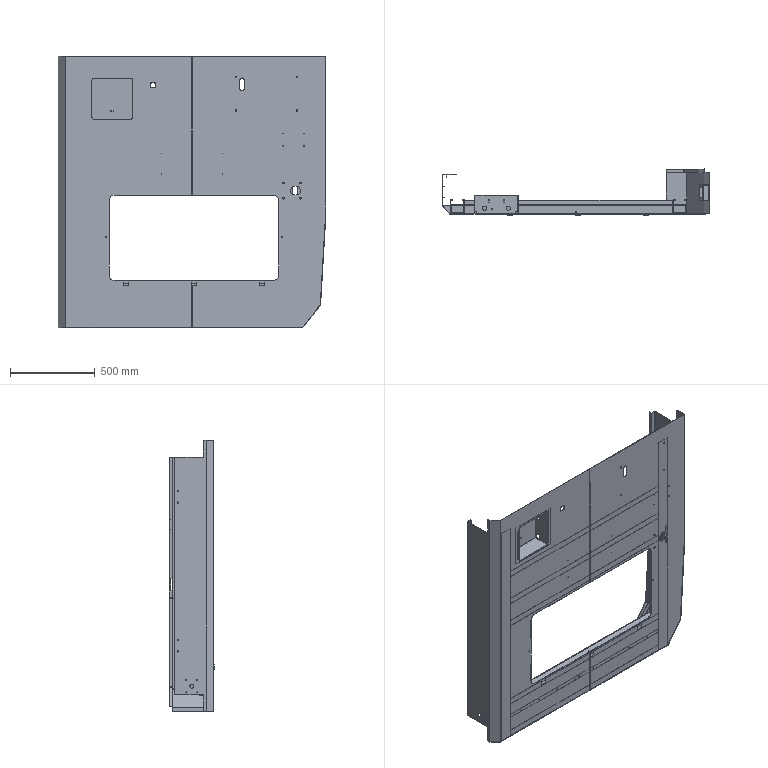Part | SolidWorks | features LocalLPattern 1 | 32 solids | 1267 faces | box 1580 x 269.314 x 1600 mm | volume 10508370 mm3 | plane 644 | cylinder 587 | cone 16 | torus 16 | spline 4 | commonest cylinder face diameters 4.2 x110 6 x95 3.3 x70 0.4 x55 3.4 x29 4.4 x26